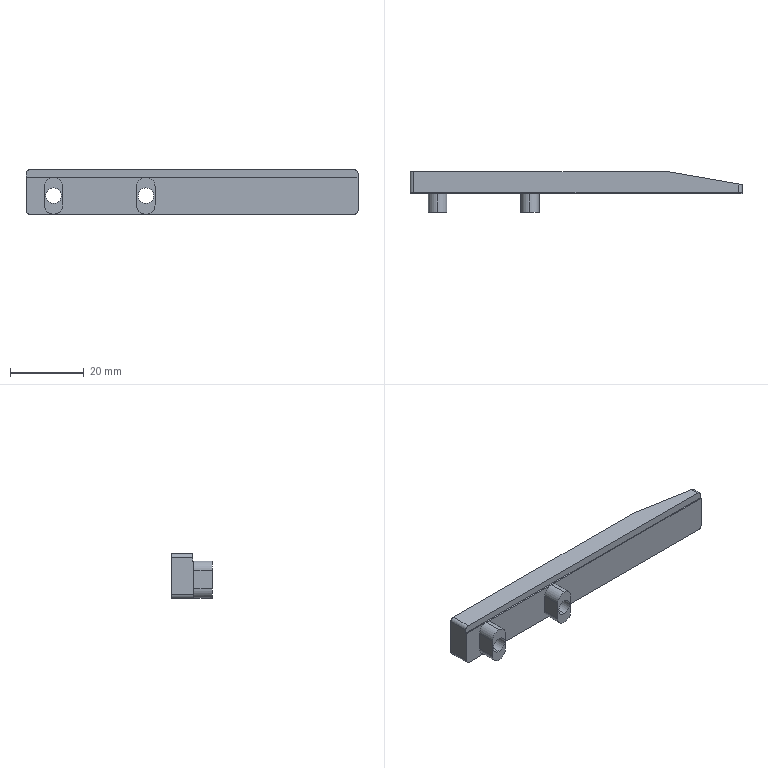Part | STEP file | 10000020548swp000-1 | 1 solid | 37 faces | box 90 x 11 x 12 mm | volume 5809 mm3 | plane 19 | cylinder 18 | commonest cylinder face diameters 5 x6 2 x4 4.2 x4 8 x4
STEP:
#1=CARTESIAN_POINT('',(7.5,1.4,-5.));
#2=VERTEX_POINT('',#1);
#3=CARTESIAN_POINT('',(7.5,1.4,3.));
#4=VERTEX_POINT('',#3);
#5=CARTESIAN_POINT('',(7.5,1.4,-1.));
#6=DIRECTION('',(0.,1.,0.));
#7=DIRECTION('',(0.,0.,1.));
#8=AXIS2_PLACEMENT_3D('',#5,#6,#7);
#9=CIRCLE('',#8,4.);
#10=EDGE_CURVE('',#2,#4,#9,.T.);
#11=ORIENTED_EDGE('',*,*,#10,.F.);
#12=CARTESIAN_POINT('',(7.5,6.,-5.));
#13=VERTEX_POINT('',#12);
#14=CARTESIAN_POINT('',(7.5,6.,-5.));
#15=DIRECTION('',(0.,1.,0.));
#16=VECTOR('',#15,1000.);
#17=LINE('',#14,#16);
#18=EDGE_CURVE('',#2,#13,#17,.T.);
#19=ORIENTED_EDGE('',*,*,#18,.T.);
#20=CARTESIAN_POINT('',(7.5,6.,3.));
#21=VERTEX_POINT('',#20);
#22=CARTESIAN_POINT('',(7.5,6.,-1.));
#23=DIRECTION('',(0.,1.,0.));
#24=DIRECTION('',(0.,0.,1.));
#25=AXIS2_PLACEMENT_3D('',#22,#23,#24);
#26=CIRCLE('',#25,4.);
#27=EDGE_CURVE('',#13,#21,#26,.T.);
#28=ORIENTED_EDGE('',*,*,#27,.T.);
#29=CARTESIAN_POINT('',(7.5,6.,3.));
#30=DIRECTION('',(0.,1.,0.));
#31=VECTOR('',#30,1000.);
#32=LINE('',#29,#31);
#33=EDGE_CURVE('',#4,#21,#32,.T.);
#34=ORIENTED_EDGE('',*,*,#33,.F.);
#35=EDGE_LOOP('',(#11,#19,#28,#34));
#36=FACE_OUTER_BOUND('',#35,.T.);
#37=CARTESIAN_POINT('',(7.5,6.,-1.));
#38=DIRECTION('',(0.,1.,0.));
#39=DIRECTION('',(0.,0.,1.));
#40=AXIS2_PLACEMENT_3D('',#37,#38,#39);
#41=CYLINDRICAL_SURFACE('',#40,4.);
#42=ADVANCED_FACE('',(#36),#41,.F.);
#43=CARTESIAN_POINT('',(7.5,-5.,1.1));
#44=VERTEX_POINT('',#43);
#45=CARTESIAN_POINT('',(7.5,-5.,-3.1));
#46=VERTEX_POINT('',#45);
#47=CARTESIAN_POINT('',(7.5,-5.,-1.));
#48=DIRECTION('',(0.,-1.,0.));
#49=DIRECTION('',(0.,0.,-1.));
#50=AXIS2_PLACEMENT_3D('',#47,#48,#49);
#51=CIRCLE('',#50,2.1);
#52=EDGE_CURVE('',#44,#46,#51,.T.);
#53=ORIENTED_EDGE('',*,*,#52,.T.);
#54=CARTESIAN_POINT('',(7.5,1.4,-3.1));
#55=VERTEX_POINT('',#54);
#56=CARTESIAN_POINT('',(7.5,6.,-3.1));
#57=DIRECTION('',(0.,1.,0.));
#58=VECTOR('',#57,1000.);
#59=LINE('',#56,#58);
#60=EDGE_CURVE('',#46,#55,#59,.T.);
#61=ORIENTED_EDGE('',*,*,#60,.T.);
#62=CARTESIAN_POINT('',(7.5,1.4,1.1));
#63=VERTEX_POINT('',#62);
#64=CARTESIAN_POINT('',(7.5,1.4,-1.));
#65=DIRECTION('',(0.,1.,0.));
#66=DIRECTION('',(0.,0.,1.));
#67=AXIS2_PLACEMENT_3D('',#64,#65,#66);
#68=CIRCLE('',#67,2.1);
#69=EDGE_CURVE('',#55,#63,#68,.T.);
#70=ORIENTED_EDGE('',*,*,#69,.T.);
#71=CARTESIAN_POINT('',(7.5,6.,1.1));
#72=DIRECTION('',(0.,1.,0.));
#73=VECTOR('',#72,1000.);
#74=LINE('',#71,#73);
#75=EDGE_CURVE('',#44,#63,#74,.T.);
#76=ORIENTED_EDGE('',*,*,#75,.F.);
#77=EDGE_LOOP('',(#53,#61,#70,#76));
#78=FACE_OUTER_BOUND('',#77,.T.);
#79=CARTESIAN_POINT('',(7.5,6.,-1.));
#80=DIRECTION('',(0.,1.,0.));
#81=DIRECTION('',(0.,0.,1.));
#82=AXIS2_PLACEMENT_3D('',#79,#80,#81);
#83=CYLINDRICAL_SURFACE('',#82,2.1);
#84=ADVANCED_FACE('',(#78),#83,.F.);
#85=CARTESIAN_POINT('',(32.5,1.4,-5.));
#86=VERTEX_POINT('',#85);
#87=CARTESIAN_POINT('',(32.5,1.4,3.));
#88=VERTEX_POINT('',#87);
#89=CARTESIAN_POINT('',(32.5,1.4,-1.));
#90=DIRECTION('',(0.,1.,0.));
#91=DIRECTION('',(0.,0.,1.));
#92=AXIS2_PLACEMENT_3D('',#89,#90,#91);
#93=CIRCLE('',#92,4.);
#94=EDGE_CURVE('',#86,#88,#93,.T.);
#95=ORIENTED_EDGE('',*,*,#94,.F.);
#96=CARTESIAN_POINT('',(32.5,6.,-5.));
#97=VERTEX_POINT('',#96);
#98=CARTESIAN_POINT('',(32.5,6.,-5.));
#99=DIRECTION('',(0.,1.,0.));
#100=VECTOR('',#99,1000.);
#101=LINE('',#98,#100);
#102=EDGE_CURVE('',#86,#97,#101,.T.);
#103=ORIENTED_EDGE('',*,*,#102,.T.);
#104=CARTESIAN_POINT('',(32.5,6.,3.));
#105=VERTEX_POINT('',#104);
#106=CARTESIAN_POINT('',(32.5,6.,-1.));
#107=DIRECTION('',(0.,1.,0.));
#108=DIRECTION('',(0.,0.,1.));
#109=AXIS2_PLACEMENT_3D('',#106,#107,#108);
#110=CIRCLE('',#109,4.);
#111=EDGE_CURVE('',#97,#105,#110,.T.);
#112=ORIENTED_EDGE('',*,*,#111,.T.);
#113=CARTESIAN_POINT('',(32.5,6.,3.));
#114=DIRECTION('',(0.,1.,0.));
#115=VECTOR('',#114,1000.);
#116=LINE('',#113,#115);
#117=EDGE_CURVE('',#88,#105,#116,.T.);
#118=ORIENTED_EDGE('',*,*,#117,.F.);
#119=EDGE_LOOP('',(#95,#103,#112,#118));
#120=FACE_OUTER_BOUND('',#119,.T.);
#121=CARTESIAN_POINT('',(32.5,6.,-1.));
#122=DIRECTION('',(0.,1.,0.));
#123=DIRECTION('',(0.,0.,1.));
#124=AXIS2_PLACEMENT_3D('',#121,#122,#123);
#125=CYLINDRICAL_SURFACE('',#124,4.);
#126=ADVANCED_FACE('',(#120),#125,.F.);
#127=CARTESIAN_POINT('',(32.5,-5.,1.1));
#128=VERTEX_POINT('',#127);
#129=CARTESIAN_POINT('',(32.5,-5.,-3.1));
#130=VERTEX_POINT('',#129);
#131=CARTESIAN_POINT('',(32.5,-5.,-1.));
#132=DIRECTION('',(0.,-1.,0.));
#133=DIRECTION('',(0.,0.,-1.));
#134=AXIS2_PLACEMENT_3D('',#131,#132,#133);
#135=CIRCLE('',#134,2.1);
#136=EDGE_CURVE('',#128,#130,#135,.T.);
#137=ORIENTED_EDGE('',*,*,#136,.T.);
#138=CARTESIAN_POINT('',(32.5,1.4,-3.1));
#139=VERTEX_POINT('',#138);
#140=CARTESIAN_POINT('',(32.5,6.,-3.1));
#141=DIRECTION('',(0.,1.,0.));
#142=VECTOR('',#141,1000.);
#143=LINE('',#140,#142);
#144=EDGE_CURVE('',#130,#139,#143,.T.);
#145=ORIENTED_EDGE('',*,*,#144,.T.);
#146=CARTESIAN_POINT('',(32.5,1.4,1.1));
#147=VERTEX_POINT('',#146);
#148=CARTESIAN_POINT('',(32.5,1.4,-1.));
#149=DIRECTION('',(0.,1.,0.));
#150=DIRECTION('',(0.,0.,1.));
#151=AXIS2_PLACEMENT_3D('',#148,#149,#150);
#152=CIRCLE('',#151,2.1);
#153=EDGE_CURVE('',#139,#147,#152,.T.);
#154=ORIENTED_EDGE('',*,*,#153,.T.);
#155=CARTESIAN_POINT('',(32.5,6.,1.1));
#156=DIRECTION('',(0.,1.,0.));
#157=VECTOR('',#156,1000.);
#158=LINE('',#155,#157);
#159=EDGE_CURVE('',#128,#147,#158,.T.);
#160=ORIENTED_EDGE('',*,*,#159,.F.);
#161=EDGE_LOOP('',(#137,#145,#154,#160));
#162=FACE_OUTER_BOUND('',#161,.T.);
#163=CARTESIAN_POINT('',(32.5,6.,-1.));
#164=DIRECTION('',(0.,1.,0.));
#165=DIRECTION('',(0.,0.,1.));
#166=AXIS2_PLACEMENT_3D('',#163,#164,#165);
#167=CYLINDRICAL_SURFACE('',#166,2.1);
#168=ADVANCED_FACE('',(#162),#167,.F.);
#169=CARTESIAN_POINT('',(32.5,-5.,4.));
#170=VERTEX_POINT('',#169);
#171=CARTESIAN_POINT('',(30.,-5.,1.5));
#172=VERTEX_POINT('',#171);
#173=CARTESIAN_POINT('',(32.5,-5.,1.5));
#174=DIRECTION('',(0.,-1.,0.));
#175=DIRECTION('',(0.,0.,-1.));
#176=AXIS2_PLACEMENT_3D('',#173,#174,#175);
#177=CIRCLE('',#176,2.5);
#178=EDGE_CURVE('',#170,#172,#177,.T.);
#179=ORIENTED_EDGE('',*,*,#178,.F.);
#180=CARTESIAN_POINT('',(32.5,0.,4.));
#181=VERTEX_POINT('',#180);
#182=CARTESIAN_POINT('',(32.5,-5.,4.));
#183=DIRECTION('',(0.,1.,0.));
#184=VECTOR('',#183,1000.);
#185=LINE('',#182,#184);
#186=EDGE_CURVE('',#170,#181,#185,.T.);
#187=ORIENTED_EDGE('',*,*,#186,.T.);
#188=CARTESIAN_POINT('',(30.,0.,1.5));
#189=VERTEX_POINT('',#188);
#190=CARTESIAN_POINT('',(32.5,0.,1.5));
#191=DIRECTION('',(0.,-1.,0.));
#192=DIRECTION('',(0.,0.,-1.));
#193=AXIS2_PLACEMENT_3D('',#190,#191,#192);
#194=CIRCLE('',#193,2.5);
#195=EDGE_CURVE('',#181,#189,#194,.T.);
#196=ORIENTED_EDGE('',*,*,#195,.T.);
#197=CARTESIAN_POINT('',(30.,-5.,1.5));
#198=DIRECTION('',(0.,1.,0.));
#199=VECTOR('',#198,1000.);
#200=LINE('',#197,#199);
#201=EDGE_CURVE('',#172,#189,#200,.T.);
#202=ORIENTED_EDGE('',*,*,#201,.F.);
#203=EDGE_LOOP('',(#179,#187,#196,#202));
#204=FACE_OUTER_BOUND('',#203,.T.);
#205=CARTESIAN_POINT('',(32.5,-5.,1.5));
#206=DIRECTION('',(0.,1.,0.));
#207=DIRECTION('',(0.,0.,1.));
#208=AXIS2_PLACEMENT_3D('',#205,#206,#207);
#209=CYLINDRICAL_SURFACE('',#208,2.5);
#210=ADVANCED_FACE('',(#204),#209,.T.);
#211=CARTESIAN_POINT('',(7.5,-5.,4.));
#212=VERTEX_POINT('',#211);
#213=CARTESIAN_POINT('',(5.,-5.,1.5));
#214=VERTEX_POINT('',#213);
#215=CARTESIAN_POINT('',(7.5,-5.,1.5));
#216=DIRECTION('',(0.,-1.,0.));
#217=DIRECTION('',(0.,0.,-1.));
#218=AXIS2_PLACEMENT_3D('',#215,#216,#217);
#219=CIRCLE('',#218,2.5);
#220=EDGE_CURVE('',#212,#214,#219,.T.);
#221=ORIENTED_EDGE('',*,*,#220,.F.);
#222=CARTESIAN_POINT('',(7.5,0.,4.));
#223=VERTEX_POINT('',#222);
#224=CARTESIAN_POINT('',(7.5,-5.,4.));
#225=DIRECTION('',(0.,1.,0.));
#226=VECTOR('',#225,1000.);
#227=LINE('',#224,#226);
#228=EDGE_CURVE('',#212,#223,#227,.T.);
#229=ORIENTED_EDGE('',*,*,#228,.T.);
#230=CARTESIAN_POINT('',(5.,0.,1.5));
#231=VERTEX_POINT('',#230);
#232=CARTESIAN_POINT('',(7.5,0.,1.5));
#233=DIRECTION('',(0.,-1.,0.));
#234=DIRECTION('',(0.,0.,-1.));
#235=AXIS2_PLACEMENT_3D('',#232,#233,#234);
#236=CIRCLE('',#235,2.5);
#237=EDGE_CURVE('',#223,#231,#236,.T.);
#238=ORIENTED_EDGE('',*,*,#237,.T.);
#239=CARTESIAN_POINT('',(5.,-5.,1.5));
#240=DIRECTION('',(0.,1.,0.));
#241=VECTOR('',#240,1000.);
#242=LINE('',#239,#241);
#243=EDGE_CURVE('',#214,#231,#242,.T.);
#244=ORIENTED_EDGE('',*,*,#243,.F.);
#245=EDGE_LOOP('',(#221,#229,#238,#244));
#246=FACE_OUTER_BOUND('',#245,.T.);
#247=CARTESIAN_POINT('',(7.5,-5.,1.5));
#248=DIRECTION('',(0.,1.,0.));
#249=DIRECTION('',(0.,0.,1.));
#250=AXIS2_PLACEMENT_3D('',#247,#248,#249);
#251=CYLINDRICAL_SURFACE('',#250,2.5);
#252=ADVANCED_FACE('',(#246),#251,.T.);
#253=CARTESIAN_POINT('',(32.5,0.,-6.));
#254=VERTEX_POINT('',#253);
#255=CARTESIAN_POINT('',(89.,0.,-6.));
#256=VERTEX_POINT('',#255);
#257=CARTESIAN_POINT('',(0.,0.,-6.));
#258=DIRECTION('',(1.,0.,0.));
#259=VECTOR('',#258,1000.);
#260=LINE('',#257,#259);
#261=EDGE_CURVE('',#254,#256,#260,.T.);
#262=ORIENTED_EDGE('',*,*,#261,.T.);
#263=CARTESIAN_POINT('',(90.,0.,-5.));
#264=VERTEX_POINT('',#263);
#265=CARTESIAN_POINT('',(89.,0.,-5.));
#266=DIRECTION('',(0.,-1.,0.));
#267=DIRECTION('',(0.,0.,1.));
#268=AXIS2_PLACEMENT_3D('',#265,#266,#267);
#269=CIRCLE('',#268,1.);
#270=EDGE_CURVE('',#256,#264,#269,.T.);
#271=ORIENTED_EDGE('',*,*,#270,.T.);
#272=CARTESIAN_POINT('',(90.,0.,4.));
#273=VERTEX_POINT('',#272);
#274=CARTESIAN_POINT('',(90.,0.,6.));
#275=DIRECTION('',(0.,0.,-1.));
#276=VECTOR('',#275,1000.);
#277=LINE('',#274,#276);
#278=EDGE_CURVE('',#273,#264,#277,.T.);
#279=ORIENTED_EDGE('',*,*,#278,.F.);
#280=CARTESIAN_POINT('',(90.,0.,4.));
#281=DIRECTION('',(1.,0.,0.));
#282=VECTOR('',#281,1000.);
#283=LINE('',#280,#282);
#284=EDGE_CURVE('',#181,#273,#283,.T.);
#285=ORIENTED_EDGE('',*,*,#284,.F.);
#286=CARTESIAN_POINT('',(35.,0.,1.5));
#287=VERTEX_POINT('',#286);
#288=CARTESIAN_POINT('',(32.5,0.,1.5));
#289=DIRECTION('',(0.,-1.,0.));
#290=DIRECTION('',(0.,0.,-1.));
#291=AXIS2_PLACEMENT_3D('',#288,#289,#290);
#292=CIRCLE('',#291,2.5);
#293=EDGE_CURVE('',#287,#181,#292,.T.);
#294=ORIENTED_EDGE('',*,*,#293,.F.);
#295=CARTESIAN_POINT('',(35.,0.,-3.5));
#296=VERTEX_POINT('',#295);
#297=CARTESIAN_POINT('',(35.,0.,1.5));
#298=DIRECTION('',(0.,0.,1.));
#299=VECTOR('',#298,1000.);
#300=LINE('',#297,#299);
#301=EDGE_CURVE('',#296,#287,#300,.T.);
#302=ORIENTED_EDGE('',*,*,#301,.F.);
#303=CARTESIAN_POINT('',(32.5,0.,-3.5));
#304=DIRECTION('',(0.,-1.,0.));
#305=DIRECTION('',(0.,0.,-1.));
#306=AXIS2_PLACEMENT_3D('',#303,#304,#305);
#307=CIRCLE('',#306,2.5);
#308=EDGE_CURVE('',#254,#296,#307,.T.);
#309=ORIENTED_EDGE('',*,*,#308,.F.);
#310=EDGE_LOOP('',(#262,#271,#279,#285,#294,#302,#309));
#311=FACE_OUTER_BOUND('',#310,.T.);
#312=CARTESIAN_POINT('',(0.,0.,6.));
#313=DIRECTION('',(0.,1.,0.));
#314=DIRECTION('',(0.,0.,1.));
#315=AXIS2_PLACEMENT_3D('',#312,#313,#314);
#316=PLANE('',#315);
#317=ADVANCED_FACE('',(#311),#316,.F.);
#318=ORIENTED_EDGE('',*,*,#195,.F.);
#319=CARTESIAN_POINT('',(90.,0.,4.));
#320=DIRECTION('',(1.,0.,0.));
#321=VECTOR('',#320,1000.);
#322=LINE('',#319,#321);
#323=EDGE_CURVE('',#223,#181,#322,.T.);
#324=ORIENTED_EDGE('',*,*,#323,.F.);
#325=CARTESIAN_POINT('',(10.,0.,1.5));
#326=VERTEX_POINT('',#325);
#327=CARTESIAN_POINT('',(7.5,0.,1.5));
#328=DIRECTION('',(0.,-1.,0.));
#329=DIRECTION('',(0.,0.,-1.));
#330=AXIS2_PLACEMENT_3D('',#327,#328,#329);
#331=CIRCLE('',#330,2.5);
#332=EDGE_CURVE('',#326,#223,#331,.T.);
#333=ORIENTED_EDGE('',*,*,#332,.F.);
#334=CARTESIAN_POINT('',(10.,0.,-3.5));
#335=VERTEX_POINT('',#334);
#336=CARTESIAN_POINT('',(10.,0.,1.5));
#337=DIRECTION('',(0.,0.,1.));
#338=VECTOR('',#337,1000.);
#339=LINE('',#336,#338);
#340=EDGE_CURVE('',#335,#326,#339,.T.);
#341=ORIENTED_EDGE('',*,*,#340,.F.);
#342=CARTESIAN_POINT('',(7.5,0.,-6.));
#343=VERTEX_POINT('',#342);
#344=CARTESIAN_POINT('',(7.5,0.,-3.5));
#345=DIRECTION('',(0.,-1.,0.));
#346=DIRECTION('',(0.,0.,-1.));
#347=AXIS2_PLACEMENT_3D('',#344,#345,#346);
#348=CIRCLE('',#347,2.5);
#349=EDGE_CURVE('',#343,#335,#348,.T.);
#350=ORIENTED_EDGE('',*,*,#349,.F.);
#351=CARTESIAN_POINT('',(0.,0.,-6.));
#352=DIRECTION('',(1.,0.,0.));
#353=VECTOR('',#352,1000.);
#354=LINE('',#351,#353);
#355=EDGE_CURVE('',#343,#254,#354,.T.);
#356=ORIENTED_EDGE('',*,*,#355,.T.);
#357=CARTESIAN_POINT('',(30.,0.,-3.5));
#358=VERTEX_POINT('',#357);
#359=CARTESIAN_POINT('',(32.5,0.,-3.5));
#360=DIRECTION('',(0.,-1.,0.));
#361=DIRECTION('',(0.,0.,-1.));
#362=AXIS2_PLACEMENT_3D('',#359,#360,#361);
#363=CIRCLE('',#362,2.5);
#364=EDGE_CURVE('',#358,#254,#363,.T.);
#365=ORIENTED_EDGE('',*,*,#364,.F.);
#366=CARTESIAN_POINT('',(30.,0.,1.5));
#367=DIRECTION('',(0.,0.,-1.));
#368=VECTOR('',#367,1000.);
#369=LINE('',#366,#368);
#370=EDGE_CURVE('',#189,#358,#369,.T.);
#371=ORIENTED_EDGE('',*,*,#370,.F.);
#372=EDGE_LOOP('',(#318,#324,#333,#341,#350,#356,#365,#371));
#373=FACE_OUTER_BOUND('',#372,.T.);
#374=CARTESIAN_POINT('',(0.,0.,6.));
#375=DIRECTION('',(0.,1.,0.));
#376=DIRECTION('',(0.,0.,1.));
#377=AXIS2_PLACEMENT_3D('',#374,#375,#376);
#378=PLANE('',#377);
#379=ADVANCED_FACE('',(#373),#378,.F.);
#380=CARTESIAN_POINT('',(0.,0.,4.));
#381=VERTEX_POINT('',#380);
#382=CARTESIAN_POINT('',(0.,0.,-5.));
#383=VERTEX_POINT('',#382);
#384=CARTESIAN_POINT('',(0.,0.,6.));
#385=DIRECTION('',(0.,0.,-1.));
#386=VECTOR('',#385,1000.);
#387=LINE('',#384,#386);
#388=EDGE_CURVE('',#381,#383,#387,.T.);
#389=ORIENTED_EDGE('',*,*,#388,.T.);
#390=CARTESIAN_POINT('',(1.,0.,-6.));
#391=VERTEX_POINT('',#390);
#392=CARTESIAN_POINT('',(1.,0.,-5.));
#393=DIRECTION('',(0.,-1.,0.));
#394=DIRECTION('',(0.,0.,1.));
#395=AXIS2_PLACEMENT_3D('',#392,#393,#394);
#396=CIRCLE('',#395,1.);
#397=EDGE_CURVE('',#383,#391,#396,.T.);
#398=ORIENTED_EDGE('',*,*,#397,.T.);
#399=CARTESIAN_POINT('',(0.,0.,-6.));
#400=DIRECTION('',(1.,0.,0.));
#401=VECTOR('',#400,1000.);
#402=LINE('',#399,#401);
#403=EDGE_CURVE('',#391,#343,#402,.T.);
#404=ORIENTED_EDGE('',*,*,#403,.T.);
#405=CARTESIAN_POINT('',(5.,0.,-3.5));
#406=VERTEX_POINT('',#405);
#407=CARTESIAN_POINT('',(7.5,0.,-3.5));
#408=DIRECTION('',(0.,-1.,0.));
#409=DIRECTION('',(0.,0.,-1.));
#410=AXIS2_PLACEMENT_3D('',#407,#408,#409);
#411=CIRCLE('',#410,2.5);
#412=EDGE_CURVE('',#406,#343,#411,.T.);
#413=ORIENTED_EDGE('',*,*,#412,.F.);
#414=CARTESIAN_POINT('',(5.,0.,1.5));
#415=DIRECTION('',(0.,0.,-1.));
#416=VECTOR('',#415,1000.);
#417=LINE('',#414,#416);
#418=EDGE_CURVE('',#231,#406,#417,.T.);
#419=ORIENTED_EDGE('',*,*,#418,.F.);
#420=ORIENTED_EDGE('',*,*,#237,.F.);
#421=CARTESIAN_POINT('',(90.,0.,4.));
#422=DIRECTION('',(1.,0.,0.));
#423=VECTOR('',#422,1000.);
#424=LINE('',#421,#423);
#425=EDGE_CURVE('',#381,#223,#424,.T.);
#426=ORIENTED_EDGE('',*,*,#425,.F.);
#427=EDGE_LOOP('',(#389,#398,#404,#413,#419,#420,#426));
#428=FACE_OUTER_BOUND('',#427,.T.);
#429=CARTESIAN_POINT('',(0.,0.,6.));
#430=DIRECTION('',(0.,1.,0.));
#431=DIRECTION('',(0.,0.,1.));
#432=AXIS2_PLACEMENT_3D('',#429,#430,#431);
#433=PLANE('',#432);
#434=ADVANCED_FACE('',(#428),#433,.F.);
#435=CARTESIAN_POINT('',(0.,6.,5.));
#436=VERTEX_POINT('',#435);
#437=CARTESIAN_POINT('',(0.,6.,-5.));
#438=VERTEX_POINT('',#437);
#439=CARTESIAN_POINT('',(0.,6.,6.));
#440=DIRECTION('',(0.,0.,-1.));
#441=VECTOR('',#440,1000.);
#442=LINE('',#439,#441);
#443=EDGE_CURVE('',#436,#438,#442,.T.);
#444=ORIENTED_EDGE('',*,*,#443,.T.);
#445=CARTESIAN_POINT('',(0.,0.,-5.));
#446=DIRECTION('',(0.,-1.,0.));
#447=VECTOR('',#446,1000.);
#448=LINE('',#445,#447);
#449=EDGE_CURVE('',#438,#383,#448,.T.);
#450=ORIENTED_EDGE('',*,*,#449,.T.);
#451=ORIENTED_EDGE('',*,*,#388,.F.);
#452=CARTESIAN_POINT('',(0.,0.3,4.));
#453=VERTEX_POINT('',#452);
#454=CARTESIAN_POINT('',(0.,0.,4.));
#455=DIRECTION('',(0.,-1.,0.));
#456=VECTOR('',#455,1000.);
#457=LINE('',#454,#456);
#458=EDGE_CURVE('',#453,#381,#457,.T.);
#459=ORIENTED_EDGE('',*,*,#458,.F.);
#460=CARTESIAN_POINT('',(0.,0.3,5.));
#461=VERTEX_POINT('',#460);
#462=CARTESIAN_POINT('',(0.,0.3,4.));
#463=DIRECTION('',(0.,0.,1.));
#464=VECTOR('',#463,1000.);
#465=LINE('',#462,#464);
#466=EDGE_CURVE('',#453,#461,#465,.T.);
#467=ORIENTED_EDGE('',*,*,#466,.T.);
#468=CARTESIAN_POINT('',(0.,0.,5.));
#469=DIRECTION('',(0.,1.,0.));
#470=VECTOR('',#469,1000.);
#471=LINE('',#468,#470);
#472=EDGE_CURVE('',#461,#436,#471,.T.);
#473=ORIENTED_EDGE('',*,*,#472,.T.);
#474=EDGE_LOOP('',(#444,#450,#451,#459,#467,#473));
#475=FACE_OUTER_BOUND('',#474,.T.);
#476=CARTESIAN_POINT('',(0.,0.,6.));
#477=DIRECTION('',(1.,0.,0.));
#478=DIRECTION('',(0.,0.,-1.));
#479=AXIS2_PLACEMENT_3D('',#476,#477,#478);
#480=PLANE('',#479);
#481=ADVANCED_FACE('',(#475),#480,.F.);
#482=ORIENTED_EDGE('',*,*,#278,.T.);
#483=CARTESIAN_POINT('',(90.,2.5,-5.));
#484=VERTEX_POINT('',#483);
#485=CARTESIAN_POINT('',(90.,2.5,-5.));
#486=DIRECTION('',(0.,1.,0.));
#487=VECTOR('',#486,1000.);
#488=LINE('',#485,#487);
#489=EDGE_CURVE('',#264,#484,#488,.T.);
#490=ORIENTED_EDGE('',*,*,#489,.T.);
#491=CARTESIAN_POINT('',(90.,2.5,5.));
#492=VERTEX_POINT('',#491);
#493=CARTESIAN_POINT('',(90.,2.5,6.));
#494=DIRECTION('',(0.,0.,-1.));
#495=VECTOR('',#494,1000.);
#496=LINE('',#493,#495);
#497=EDGE_CURVE('',#492,#484,#496,.T.);
#498=ORIENTED_EDGE('',*,*,#497,.F.);
#499=CARTESIAN_POINT('',(90.,0.3,5.));
#500=VERTEX_POINT('',#499);
#501=CARTESIAN_POINT('',(90.,0.,5.));
#502=DIRECTION('',(0.,-1.,0.));
#503=VECTOR('',#502,1000.);
#504=LINE('',#501,#503);
#505=EDGE_CURVE('',#492,#500,#504,.T.);
#506=ORIENTED_EDGE('',*,*,#505,.T.);
#507=CARTESIAN_POINT('',(90.,0.3,4.));
#508=VERTEX_POINT('',#507);
#509=CARTESIAN_POINT('',(90.,0.3,4.));
#510=DIRECTION('',(0.,0.,1.));
#511=VECTOR('',#510,1000.);
#512=LINE('',#509,#511);
#513=EDGE_CURVE('',#508,#500,#512,.T.);
#514=ORIENTED_EDGE('',*,*,#513,.F.);
#515=CARTESIAN_POINT('',(90.,0.,4.));
#516=DIRECTION('',(0.,1.,0.));
#517=VECTOR('',#516,1000.);
#518=LINE('',#515,#517);
#519=EDGE_CURVE('',#273,#508,#518,.T.);
#520=ORIENTED_EDGE('',*,*,#519,.F.);
#521=EDGE_LOOP('',(#482,#490,#498,#506,#514,#520));
#522=FACE_OUTER_BOUND('',#521,.T.);
#523=CARTESIAN_POINT('',(90.,0.,6.));
#524=DIRECTION('',(-1.,0.,0.));
#525=DIRECTION('',(0.,0.,1.));
#526=AXIS2_PLACEMENT_3D('',#523,#524,#525);
#527=PLANE('',#526);
#528=ADVANCED_FACE('',(#522),#527,.F.);
#529=ORIENTED_EDGE('',*,*,#497,.T.);
#530=CARTESIAN_POINT('',(89.,2.675,-6.));
#531=VERTEX_POINT('',#530);
#532=CARTESIAN_POINT('',(90.,2.5,-5.));
#533=CARTESIAN_POINT('',(90.,2.5,-5.586));
#534=CARTESIAN_POINT('',(89.586,2.572,-6.));
#535=CARTESIAN_POINT('',(89.,2.675,-6.));
#536=(BOUNDED_CURVE()B_SPLINE_CURVE(3,(#532,#533,#534,#535),.UNSPECIFIED.,.F.,.F.)B_SPLINE_CURVE_WITH_KNOTS((4,4),(0.,1.571),.UNSPECIFIED.)CURVE()GEOMETRIC_REPRESENTATION_ITEM()RATIONAL_B_SPLINE_CURVE((1.,0.8047,0.8047,1.))REPRESENTATION_ITEM(''));
#537=EDGE_CURVE('',#484,#531,#536,.T.);
#538=ORIENTED_EDGE('',*,*,#537,.T.);
#539=CARTESIAN_POINT('',(70.,6.,-6.));
#540=VERTEX_POINT('',#539);
#541=CARTESIAN_POINT('',(90.,2.5,-6.));
#542=DIRECTION('',(-0.985,0.1724,0.));
#543=VECTOR('',#542,1000.);
#544=LINE('',#541,#543);
#545=EDGE_CURVE('',#531,#540,#544,.T.);
#546=ORIENTED_EDGE('',*,*,#545,.T.);
#547=CARTESIAN_POINT('',(70.,6.,6.));
#548=VERTEX_POINT('',#547);
#549=CARTESIAN_POINT('',(70.,6.,6.));
#550=DIRECTION('',(0.,0.,-1.));
#551=VECTOR('',#550,1000.);
#552=LINE('',#549,#551);
#553=EDGE_CURVE('',#548,#540,#552,.T.);
#554=ORIENTED_EDGE('',*,*,#553,.F.);
#555=CARTESIAN_POINT('',(89.,2.675,6.));
#556=VERTEX_POINT('',#555);
#557=CARTESIAN_POINT('',(90.,2.5,6.));
#558=DIRECTION('',(-0.985,0.1724,0.));
#559=VECTOR('',#558,1000.);
#560=LINE('',#557,#559);
#561=EDGE_CURVE('',#556,#548,#560,.T.);
#562=ORIENTED_EDGE('',*,*,#561,.F.);
#563=CARTESIAN_POINT('',(89.,2.675,6.));
#564=CARTESIAN_POINT('',(89.586,2.572,6.));
#565=CARTESIAN_POINT('',(90.,2.5,5.586));
#566=CARTESIAN_POINT('',(90.,2.5,5.));
#567=(BOUNDED_CURVE()B_SPLINE_CURVE(3,(#563,#564,#565,#566),.UNSPECIFIED.,.F.,.F.)B_SPLINE_CURVE_WITH_KNOTS((4,4),(1.571,3.142),.UNSPECIFIED.)CURVE()GEOMETRIC_REPRESENTATION_ITEM()RATIONAL_B_SPLINE_CURVE((1.,0.8047,0.8047,1.))REPRESENTATION_ITEM(''));
#568=EDGE_CURVE('',#556,#492,#567,.T.);
#569=ORIENTED_EDGE('',*,*,#568,.T.);
#570=EDGE_LOOP('',(#529,#538,#546,#554,#562,#569));
#571=FACE_OUTER_BOUND('',#570,.T.);
#572=CARTESIAN_POINT('',(90.,2.5,6.));
#573=DIRECTION('',(-0.1724,-0.985,0.));
#574=DIRECTION('',(0.985,-0.1724,0.));
#575=AXIS2_PLACEMENT_3D('',#572,#573,#574);
#576=PLANE('',#575);
#577=ADVANCED_FACE('',(#571),#576,.F.);
#578=CARTESIAN_POINT('',(7.5,6.,-1.));
#579=DIRECTION('',(0.,1.,0.));
#580=DIRECTION('',(0.,0.,1.));
#581=AXIS2_PLACEMENT_3D('',#578,#579,#580);
#582=CIRCLE('',#581,4.);
#583=EDGE_CURVE('',#21,#13,#582,.T.);
#584=ORIENTED_EDGE('',*,*,#583,.F.);
#585=ORIENTED_EDGE('',*,*,#27,.F.);
#586=EDGE_LOOP('',(#584,#585));
#587=FACE_BOUND('',#586,.T.);
#588=CARTESIAN_POINT('',(32.5,6.,-1.));
#589=DIRECTION('',(0.,1.,0.));
#590=DIRECTION('',(0.,0.,1.));
#591=AXIS2_PLACEMENT_3D('',#588,#589,#590);
#592=CIRCLE('',#591,4.);
#593=EDGE_CURVE('',#105,#97,#592,.T.);
#594=ORIENTED_EDGE('',*,*,#593,.F.);
#595=ORIENTED_EDGE('',*,*,#111,.F.);
#596=EDGE_LOOP('',(#594,#595));
#597=FACE_BOUND('',#596,.T.);
#598=CARTESIAN_POINT('',(1.,6.,-6.));
#599=VERTEX_POINT('',#598);
#600=CARTESIAN_POINT('',(0.,6.,-6.));
#601=DIRECTION('',(-1.,0.,0.));
#602=VECTOR('',#601,1000.);
#603=LINE('',#600,#602);
#604=EDGE_CURVE('',#540,#599,#603,.T.);
#605=ORIENTED_EDGE('',*,*,#604,.T.);
#606=CARTESIAN_POINT('',(1.,6.,-5.));
#607=DIRECTION('',(0.,1.,0.));
#608=DIRECTION('',(0.,0.,-1.));
#609=AXIS2_PLACEMENT_3D('',#606,#607,#608);
#610=CIRCLE('',#609,1.);
#611=EDGE_CURVE('',#599,#438,#610,.T.);
#612=ORIENTED_EDGE('',*,*,#611,.T.);
#613=ORIENTED_EDGE('',*,*,#443,.F.);
#614=CARTESIAN_POINT('',(1.,6.,6.));
#615=VERTEX_POINT('',#614);
#616=CARTESIAN_POINT('',(1.,6.,5.));
#617=DIRECTION('',(0.,1.,0.));
#618=DIRECTION('',(0.,0.,-1.));
#619=AXIS2_PLACEMENT_3D('',#616,#617,#618);
#620=CIRCLE('',#619,1.);
#621=EDGE_CURVE('',#436,#615,#620,.T.);
#622=ORIENTED_EDGE('',*,*,#621,.T.);
#623=CARTESIAN_POINT('',(0.,6.,6.));
#624=DIRECTION('',(-1.,0.,0.));
#625=VECTOR('',#624,1000.);
#626=LINE('',#623,#625);
#627=EDGE_CURVE('',#548,#615,#626,.T.);
#628=ORIENTED_EDGE('',*,*,#627,.F.);
#629=ORIENTED_EDGE('',*,*,#553,.T.);
#630=EDGE_LOOP('',(#605,#612,#613,#622,#628,#629));
#631=FACE_OUTER_BOUND('',#630,.T.);
#632=CARTESIAN_POINT('',(0.,6.,6.));
#633=DIRECTION('',(0.,-1.,0.));
#634=DIRECTION('',(0.,0.,-1.));
#635=AXIS2_PLACEMENT_3D('',#632,#633,#634);
#636=PLANE('',#635);
#637=ADVANCED_FACE('',(#587,#597,#631),#636,.F.);
#638=ORIENTED_EDGE('',*,*,#627,.T.);
#639=CARTESIAN_POINT('',(1.,0.3,6.));
#640=VERTEX_POINT('',#639);
#641=CARTESIAN_POINT('',(1.,0.,6.));
#642=DIRECTION('',(0.,-1.,0.));
#643=VECTOR('',#642,1000.);
#644=LINE('',#641,#643);
#645=EDGE_CURVE('',#615,#640,#644,.T.);
#646=ORIENTED_EDGE('',*,*,#645,.T.);
#647=CARTESIAN_POINT('',(89.,0.3,6.));
#648=VERTEX_POINT('',#647);
#649=CARTESIAN_POINT('',(90.,0.3,6.));
#650=DIRECTION('',(-1.,0.,0.));
#651=VECTOR('',#650,1000.);
#652=LINE('',#649,#651);
#653=EDGE_CURVE('',#648,#640,#652,.T.);
#654=ORIENTED_EDGE('',*,*,#653,.F.);
#655=CARTESIAN_POINT('',(89.,0.,6.));
#656=DIRECTION('',(0.,1.,0.));
#657=VECTOR('',#656,1000.);
#658=LINE('',#655,#657);
#659=EDGE_CURVE('',#648,#556,#658,.T.);
#660=ORIENTED_EDGE('',*,*,#659,.T.);
#661=ORIENTED_EDGE('',*,*,#561,.T.);
#662=EDGE_LOOP('',(#638,#646,#654,#660,#661));
#663=FACE_OUTER_BOUND('',#662,.T.);
#664=CARTESIAN_POINT('',(0.,0.,6.));
#665=DIRECTION('',(0.,0.,-1.));
#666=DIRECTION('',(-1.,0.,0.));
#667=AXIS2_PLACEMENT_3D('',#664,#665,#666);
#668=PLANE('',#667);
#669=ADVANCED_FACE('',(#663),#668,.F.);
#670=ORIENTED_EDGE('',*,*,#403,.F.);
#671=CARTESIAN_POINT('',(1.,6.,-6.));
#672=DIRECTION('',(0.,1.,0.));
#673=VECTOR('',#672,1000.);
#674=LINE('',#671,#673);
#675=EDGE_CURVE('',#391,#599,#674,.T.);
#676=ORIENTED_EDGE('',*,*,#675,.T.);
#677=ORIENTED_EDGE('',*,*,#604,.F.);
#678=ORIENTED_EDGE('',*,*,#545,.F.);
#679=CARTESIAN_POINT('',(89.,0.,-6.));
#680=DIRECTION('',(0.,-1.,0.));
#681=VECTOR('',#680,1000.);
#682=LINE('',#679,#681);
#683=EDGE_CURVE('',#531,#256,#682,.T.);
#684=ORIENTED_EDGE('',*,*,#683,.T.);
#685=ORIENTED_EDGE('',*,*,#261,.F.);
#686=ORIENTED_EDGE('',*,*,#355,.F.);
#687=EDGE_LOOP('',(#670,#676,#677,#678,#684,#685,#686));
#688=FACE_OUTER_BOUND('',#687,.T.);
#689=CARTESIAN_POINT('',(0.,0.,-6.));
#690=DIRECTION('',(0.,0.,-1.));
#691=DIRECTION('',(-1.,0.,0.));
#692=AXIS2_PLACEMENT_3D('',#689,#690,#691);
#693=PLANE('',#692);
#694=ADVANCED_FACE('',(#688),#693,.T.);
#695=ORIENTED_EDGE('',*,*,#653,.T.);
#696=CARTESIAN_POINT('',(1.,0.3,5.));
#697=DIRECTION('',(0.,-1.,0.));
#698=DIRECTION('',(-1.,0.,0.));
#699=AXIS2_PLACEMENT_3D('',#696,#697,#698);
#700=CIRCLE('',#699,1.);
#701=EDGE_CURVE('',#640,#461,#700,.T.);
#702=ORIENTED_EDGE('',*,*,#701,.T.);
#703=ORIENTED_EDGE('',*,*,#466,.F.);
#704=CARTESIAN_POINT('',(90.,0.3,4.));
#705=DIRECTION('',(-1.,0.,0.));
#706=VECTOR('',#705,1000.);
#707=LINE('',#704,#706);
#708=EDGE_CURVE('',#508,#453,#707,.T.);
#709=ORIENTED_EDGE('',*,*,#708,.F.);
#710=ORIENTED_EDGE('',*,*,#513,.T.);
#711=CARTESIAN_POINT('',(89.,0.3,5.));
#712=DIRECTION('',(0.,-1.,0.));
#713=DIRECTION('',(-1.,0.,0.));
#714=AXIS2_PLACEMENT_3D('',#711,#712,#713);
#715=CIRCLE('',#714,1.);
#716=EDGE_CURVE('',#500,#648,#715,.T.);
#717=ORIENTED_EDGE('',*,*,#716,.T.);
#718=EDGE_LOOP('',(#695,#702,#703,#709,#710,#717));
#719=FACE_OUTER_BOUND('',#718,.T.);
#720=CARTESIAN_POINT('',(90.,0.3,4.));
#721=DIRECTION('',(0.,1.,0.));
#722=DIRECTION('',(-1.,0.,0.));
#723=AXIS2_PLACEMENT_3D('',#720,#721,#722);
#724=PLANE('',#723);
#725=ADVANCED_FACE('',(#719),#724,.F.);
#726=ORIENTED_EDGE('',*,*,#519,.T.);
#727=ORIENTED_EDGE('',*,*,#708,.T.);
#728=ORIENTED_EDGE('',*,*,#458,.T.);
#729=ORIENTED_EDGE('',*,*,#425,.T.);
#730=ORIENTED_EDGE('',*,*,#323,.T.);
#731=ORIENTED_EDGE('',*,*,#284,.T.);
#732=EDGE_LOOP('',(#726,#727,#728,#729,#730,#731));
#733=FACE_OUTER_BOUND('',#732,.T.);
#734=CARTESIAN_POINT('',(0.,0.,4.));
#735=DIRECTION('',(0.,0.,1.));
#736=DIRECTION('',(1.,0.,0.));
#737=AXIS2_PLACEMENT_3D('',#734,#735,#736);
#738=PLANE('',#737);
#739=ADVANCED_FACE('',(#733),#738,.T.);
#740=ORIENTED_EDGE('',*,*,#228,.F.);
#741=CARTESIAN_POINT('',(10.,-5.,1.5));
#742=VERTEX_POINT('',#741);
#743=CARTESIAN_POINT('',(7.5,-5.,1.5));
#744=DIRECTION('',(0.,-1.,0.));
#745=DIRECTION('',(0.,0.,-1.));
#746=AXIS2_PLACEMENT_3D('',#743,#744,#745);
#747=CIRCLE('',#746,2.5);
#748=EDGE_CURVE('',#742,#212,#747,.T.);
#749=ORIENTED_EDGE('',*,*,#748,.F.);
#750=CARTESIAN_POINT('',(10.,-5.,1.5));
#751=DIRECTION('',(0.,1.,0.));
#752=VECTOR('',#751,1000.);
#753=LINE('',#750,#752);
#754=EDGE_CURVE('',#742,#326,#753,.T.);
#755=ORIENTED_EDGE('',*,*,#754,.T.);
#756=ORIENTED_EDGE('',*,*,#332,.T.);
#757=EDGE_LOOP('',(#740,#749,#755,#756));
#758=FACE_OUTER_BOUND('',#757,.T.);
#759=CARTESIAN_POINT('',(7.5,-5.,1.5));
#760=DIRECTION('',(0.,1.,0.));
#761=DIRECTION('',(0.,0.,1.));
#762=AXIS2_PLACEMENT_3D('',#759,#760,#761);
#763=CYLINDRICAL_SURFACE('',#762,2.5);
#764=ADVANCED_FACE('',(#758),#763,.T.);
#765=ORIENTED_EDGE('',*,*,#418,.T.);
#766=CARTESIAN_POINT('',(5.,-5.,-3.5));
#767=VERTEX_POINT('',#766);
#768=CARTESIAN_POINT('',(5.,-5.,-3.5));
#769=DIRECTION('',(0.,1.,0.));
#770=VECTOR('',#769,1000.);
#771=LINE('',#768,#770);
#772=EDGE_CURVE('',#767,#406,#771,.T.);
#773=ORIENTED_EDGE('',*,*,#772,.F.);
#774=CARTESIAN_POINT('',(5.,-5.,1.5));
#775=DIRECTION('',(0.,0.,-1.));
#776=VECTOR('',#775,1000.);
#777=LINE('',#774,#776);
#778=EDGE_CURVE('',#214,#767,#777,.T.);
#779=ORIENTED_EDGE('',*,*,#778,.F.);
#780=ORIENTED_EDGE('',*,*,#243,.T.);
#781=EDGE_LOOP('',(#765,#773,#779,#780));
#782=FACE_OUTER_BOUND('',#781,.T.);
#783=CARTESIAN_POINT('',(5.,-5.,1.5));
#784=DIRECTION('',(1.,0.,0.));
#785=DIRECTION('',(0.,0.,-1.));
#786=AXIS2_PLACEMENT_3D('',#783,#784,#785);
#787=PLANE('',#786);
#788=ADVANCED_FACE('',(#782),#787,.F.);
#789=ORIENTED_EDGE('',*,*,#412,.T.);
#790=ORIENTED_EDGE('',*,*,#349,.T.);
#791=CARTESIAN_POINT('',(10.,-5.,-3.5));
#792=VERTEX_POINT('',#791);
#793=CARTESIAN_POINT('',(10.,-5.,-3.5));
#794=DIRECTION('',(0.,1.,0.));
#795=VECTOR('',#794,1000.);
#796=LINE('',#793,#795);
#797=EDGE_CURVE('',#792,#335,#796,.T.);
#798=ORIENTED_EDGE('',*,*,#797,.F.);
#799=CARTESIAN_POINT('',(7.5,-5.,-3.5));
#800=DIRECTION('',(0.,-1.,0.));
#801=DIRECTION('',(0.,0.,-1.));
#802=AXIS2_PLACEMENT_3D('',#799,#800,#801);
#803=CIRCLE('',#802,2.5);
#804=EDGE_CURVE('',#767,#792,#803,.T.);
#805=ORIENTED_EDGE('',*,*,#804,.F.);
#806=ORIENTED_EDGE('',*,*,#772,.T.);
#807=EDGE_LOOP('',(#789,#790,#798,#805,#806));
#808=FACE_OUTER_BOUND('',#807,.T.);
#809=CARTESIAN_POINT('',(7.5,-5.,-3.5));
#810=DIRECTION('',(0.,1.,0.));
#811=DIRECTION('',(0.,0.,1.));
#812=AXIS2_PLACEMENT_3D('',#809,#810,#811);
#813=CYLINDRICAL_SURFACE('',#812,2.5);
#814=ADVANCED_FACE('',(#808),#813,.T.);
#815=ORIENTED_EDGE('',*,*,#340,.T.);
#816=ORIENTED_EDGE('',*,*,#754,.F.);
#817=CARTESIAN_POINT('',(10.,-5.,1.5));
#818=DIRECTION('',(0.,0.,1.));
#819=VECTOR('',#818,1000.);
#820=LINE('',#817,#819);
#821=EDGE_CURVE('',#792,#742,#820,.T.);
#822=ORIENTED_EDGE('',*,*,#821,.F.);
#823=ORIENTED_EDGE('',*,*,#797,.T.);
#824=EDGE_LOOP('',(#815,#816,#822,#823));
#825=FACE_OUTER_BOUND('',#824,.T.);
#826=CARTESIAN_POINT('',(10.,-5.,1.5));
#827=DIRECTION('',(-1.,0.,0.));
#828=DIRECTION('',(0.,0.,1.));
#829=AXIS2_PLACEMENT_3D('',#826,#827,#828);
#830=PLANE('',#829);
#831=ADVANCED_FACE('',(#825),#830,.F.);
#832=ORIENTED_EDGE('',*,*,#52,.F.);
#833=CARTESIAN_POINT('',(7.5,-5.,-1.));
#834=DIRECTION('',(0.,-1.,0.));
#835=DIRECTION('',(0.,0.,-1.));
#836=AXIS2_PLACEMENT_3D('',#833,#834,#835);
#837=CIRCLE('',#836,2.1);
#838=EDGE_CURVE('',#46,#44,#837,.T.);
#839=ORIENTED_EDGE('',*,*,#838,.F.);
#840=EDGE_LOOP('',(#832,#839));
#841=FACE_BOUND('',#840,.T.);
#842=ORIENTED_EDGE('',*,*,#748,.T.);
#843=ORIENTED_EDGE('',*,*,#220,.T.);
#844=ORIENTED_EDGE('',*,*,#778,.T.);
#845=ORIENTED_EDGE('',*,*,#804,.T.);
#846=ORIENTED_EDGE('',*,*,#821,.T.);
#847=EDGE_LOOP('',(#842,#843,#844,#845,#846));
#848=FACE_OUTER_BOUND('',#847,.T.);
#849=CARTESIAN_POINT('',(7.5,-5.,1.5));
#850=DIRECTION('',(0.,-1.,0.));
#851=DIRECTION('',(0.,0.,-1.));
#852=AXIS2_PLACEMENT_3D('',#849,#850,#851);
#853=PLANE('',#852);
#854=ADVANCED_FACE('',(#841,#848),#853,.T.);
#855=ORIENTED_EDGE('',*,*,#186,.F.);
#856=CARTESIAN_POINT('',(35.,-5.,1.5));
#857=VERTEX_POINT('',#856);
#858=CARTESIAN_POINT('',(32.5,-5.,1.5));
#859=DIRECTION('',(0.,-1.,0.));
#860=DIRECTION('',(0.,0.,-1.));
#861=AXIS2_PLACEMENT_3D('',#858,#859,#860);
#862=CIRCLE('',#861,2.5);
#863=EDGE_CURVE('',#857,#170,#862,.T.);
#864=ORIENTED_EDGE('',*,*,#863,.F.);
#865=CARTESIAN_POINT('',(35.,-5.,1.5));
#866=DIRECTION('',(0.,1.,0.));
#867=VECTOR('',#866,1000.);
#868=LINE('',#865,#867);
#869=EDGE_CURVE('',#857,#287,#868,.T.);
#870=ORIENTED_EDGE('',*,*,#869,.T.);
#871=ORIENTED_EDGE('',*,*,#293,.T.);
#872=EDGE_LOOP('',(#855,#864,#870,#871));
#873=FACE_OUTER_BOUND('',#872,.T.);
#874=CARTESIAN_POINT('',(32.5,-5.,1.5));
#875=DIRECTION('',(0.,1.,0.));
#876=DIRECTION('',(0.,0.,1.));
#877=AXIS2_PLACEMENT_3D('',#874,#875,#876);
#878=CYLINDRICAL_SURFACE('',#877,2.5);
#879=ADVANCED_FACE('',(#873),#878,.T.);
#880=ORIENTED_EDGE('',*,*,#370,.T.);
#881=CARTESIAN_POINT('',(30.,-5.,-3.5));
#882=VERTEX_POINT('',#881);
#883=CARTESIAN_POINT('',(30.,-5.,-3.5));
#884=DIRECTION('',(0.,1.,0.));
#885=VECTOR('',#884,1000.);
#886=LINE('',#883,#885);
#887=EDGE_CURVE('',#882,#358,#886,.T.);
#888=ORIENTED_EDGE('',*,*,#887,.F.);
#889=CARTESIAN_POINT('',(30.,-5.,1.5));
#890=DIRECTION('',(0.,0.,-1.));
#891=VECTOR('',#890,1000.);
#892=LINE('',#889,#891);
#893=EDGE_CURVE('',#172,#882,#892,.T.);
#894=ORIENTED_EDGE('',*,*,#893,.F.);
#895=ORIENTED_EDGE('',*,*,#201,.T.);
#896=EDGE_LOOP('',(#880,#888,#894,#895));
#897=FACE_OUTER_BOUND('',#896,.T.);
#898=CARTESIAN_POINT('',(30.,-5.,1.5));
#899=DIRECTION('',(1.,0.,0.));
#900=DIRECTION('',(0.,0.,-1.));
#901=AXIS2_PLACEMENT_3D('',#898,#899,#900);
#902=PLANE('',#901);
#903=ADVANCED_FACE('',(#897),#902,.F.);
#904=ORIENTED_EDGE('',*,*,#364,.T.);
#905=ORIENTED_EDGE('',*,*,#308,.T.);
#906=CARTESIAN_POINT('',(35.,-5.,-3.5));
#907=VERTEX_POINT('',#906);
#908=CARTESIAN_POINT('',(35.,-5.,-3.5));
#909=DIRECTION('',(0.,1.,0.));
#910=VECTOR('',#909,1000.);
#911=LINE('',#908,#910);
#912=EDGE_CURVE('',#907,#296,#911,.T.);
#913=ORIENTED_EDGE('',*,*,#912,.F.);
#914=CARTESIAN_POINT('',(32.5,-5.,-3.5));
#915=DIRECTION('',(0.,-1.,0.));
#916=DIRECTION('',(0.,0.,-1.));
#917=AXIS2_PLACEMENT_3D('',#914,#915,#916);
#918=CIRCLE('',#917,2.5);
#919=EDGE_CURVE('',#882,#907,#918,.T.);
#920=ORIENTED_EDGE('',*,*,#919,.F.);
#921=ORIENTED_EDGE('',*,*,#887,.T.);
#922=EDGE_LOOP('',(#904,#905,#913,#920,#921));
#923=FACE_OUTER_BOUND('',#922,.T.);
#924=CARTESIAN_POINT('',(32.5,-5.,-3.5));
#925=DIRECTION('',(0.,1.,0.));
#926=DIRECTION('',(0.,0.,1.));
#927=AXIS2_PLACEMENT_3D('',#924,#925,#926);
#928=CYLINDRICAL_SURFACE('',#927,2.5);
#929=ADVANCED_FACE('',(#923),#928,.T.);
#930=ORIENTED_EDGE('',*,*,#301,.T.);
#931=ORIENTED_EDGE('',*,*,#869,.F.);
#932=CARTESIAN_POINT('',(35.,-5.,1.5));
#933=DIRECTION('',(0.,0.,1.));
#934=VECTOR('',#933,1000.);
#935=LINE('',#932,#934);
#936=EDGE_CURVE('',#907,#857,#935,.T.);
#937=ORIENTED_EDGE('',*,*,#936,.F.);
#938=ORIENTED_EDGE('',*,*,#912,.T.);
#939=EDGE_LOOP('',(#930,#931,#937,#938));
#940=FACE_OUTER_BOUND('',#939,.T.);
#941=CARTESIAN_POINT('',(35.,-5.,1.5));
#942=DIRECTION('',(-1.,0.,0.));
#943=DIRECTION('',(0.,0.,1.));
#944=AXIS2_PLACEMENT_3D('',#941,#942,#943);
#945=PLANE('',#944);
#946=ADVANCED_FACE('',(#940),#945,.F.);
#947=ORIENTED_EDGE('',*,*,#136,.F.);
#948=CARTESIAN_POINT('',(32.5,-5.,-1.));
#949=DIRECTION('',(0.,-1.,0.));
#950=DIRECTION('',(0.,0.,-1.));
#951=AXIS2_PLACEMENT_3D('',#948,#949,#950);
#952=CIRCLE('',#951,2.1);
#953=EDGE_CURVE('',#130,#128,#952,.T.);
#954=ORIENTED_EDGE('',*,*,#953,.F.);
#955=EDGE_LOOP('',(#947,#954));
#956=FACE_BOUND('',#955,.T.);
#957=ORIENTED_EDGE('',*,*,#863,.T.);
#958=ORIENTED_EDGE('',*,*,#178,.T.);
#959=ORIENTED_EDGE('',*,*,#893,.T.);
#960=ORIENTED_EDGE('',*,*,#919,.T.);
#961=ORIENTED_EDGE('',*,*,#936,.T.);
#962=EDGE_LOOP('',(#957,#958,#959,#960,#961));
#963=FACE_OUTER_BOUND('',#962,.T.);
#964=CARTESIAN_POINT('',(32.5,-5.,1.5));
#965=DIRECTION('',(0.,-1.,0.));
#966=DIRECTION('',(0.,0.,-1.));
#967=AXIS2_PLACEMENT_3D('',#964,#965,#966);
#968=PLANE('',#967);
#969=ADVANCED_FACE('',(#956,#963),#968,.T.);
#970=ORIENTED_EDGE('',*,*,#144,.F.);
#971=ORIENTED_EDGE('',*,*,#953,.T.);
#972=ORIENTED_EDGE('',*,*,#159,.T.);
#973=CARTESIAN_POINT('',(32.5,1.4,-1.));
#974=DIRECTION('',(0.,1.,0.));
#975=DIRECTION('',(0.,0.,1.));
#976=AXIS2_PLACEMENT_3D('',#973,#974,#975);
#977=CIRCLE('',#976,2.1);
#978=EDGE_CURVE('',#147,#139,#977,.T.);
#979=ORIENTED_EDGE('',*,*,#978,.T.);
#980=EDGE_LOOP('',(#970,#971,#972,#979));
#981=FACE_OUTER_BOUND('',#980,.T.);
#982=CARTESIAN_POINT('',(32.5,6.,-1.));
#983=DIRECTION('',(0.,1.,0.));
#984=DIRECTION('',(0.,0.,1.));
#985=AXIS2_PLACEMENT_3D('',#982,#983,#984);
#986=CYLINDRICAL_SURFACE('',#985,2.1);
#987=ADVANCED_FACE('',(#981),#986,.F.);
#988=ORIENTED_EDGE('',*,*,#978,.F.);
#989=ORIENTED_EDGE('',*,*,#153,.F.);
#990=EDGE_LOOP('',(#988,#989));
#991=FACE_BOUND('',#990,.T.);
#992=CARTESIAN_POINT('',(32.5,1.4,-1.));
#993=DIRECTION('',(0.,1.,0.));
#994=DIRECTION('',(0.,0.,1.));
#995=AXIS2_PLACEMENT_3D('',#992,#993,#994);
#996=CIRCLE('',#995,4.);
#997=EDGE_CURVE('',#88,#86,#996,.T.);
#998=ORIENTED_EDGE('',*,*,#997,.T.);
#999=ORIENTED_EDGE('',*,*,#94,.T.);
#1000=EDGE_LOOP('',(#998,#999));
#1001=FACE_OUTER_BOUND('',#1000,.T.);
#1002=CARTESIAN_POINT('',(34.6,1.4,-1.));
#1003=DIRECTION('',(0.,-1.,0.));
#1004=DIRECTION('',(0.,0.,-1.));
#1005=AXIS2_PLACEMENT_3D('',#1002,#1003,#1004);
#1006=PLANE('',#1005);
#1007=ADVANCED_FACE('',(#991,#1001),#1006,.F.);
#1008=ORIENTED_EDGE('',*,*,#102,.F.);
#1009=ORIENTED_EDGE('',*,*,#997,.F.);
#1010=ORIENTED_EDGE('',*,*,#117,.T.);
#1011=ORIENTED_EDGE('',*,*,#593,.T.);
#1012=EDGE_LOOP('',(#1008,#1009,#1010,#1011));
#1013=FACE_OUTER_BOUND('',#1012,.T.);
#1014=CARTESIAN_POINT('',(32.5,6.,-1.));
#1015=DIRECTION('',(0.,1.,0.));
#1016=DIRECTION('',(0.,0.,1.));
#1017=AXIS2_PLACEMENT_3D('',#1014,#1015,#1016);
#1018=CYLINDRICAL_SURFACE('',#1017,4.);
#1019=ADVANCED_FACE('',(#1013),#1018,.F.);
#1020=ORIENTED_EDGE('',*,*,#60,.F.);
#1021=ORIENTED_EDGE('',*,*,#838,.T.);
#1022=ORIENTED_EDGE('',*,*,#75,.T.);
#1023=CARTESIAN_POINT('',(7.5,1.4,-1.));
#1024=DIRECTION('',(0.,1.,0.));
#1025=DIRECTION('',(0.,0.,1.));
#1026=AXIS2_PLACEMENT_3D('',#1023,#1024,#1025);
#1027=CIRCLE('',#1026,2.1);
#1028=EDGE_CURVE('',#63,#55,#1027,.T.);
#1029=ORIENTED_EDGE('',*,*,#1028,.T.);
#1030=EDGE_LOOP('',(#1020,#1021,#1022,#1029));
#1031=FACE_OUTER_BOUND('',#1030,.T.);
#1032=CARTESIAN_POINT('',(7.5,6.,-1.));
#1033=DIRECTION('',(0.,1.,0.));
#1034=DIRECTION('',(0.,0.,1.));
#1035=AXIS2_PLACEMENT_3D('',#1032,#1033,#1034);
#1036=CYLINDRICAL_SURFACE('',#1035,2.1);
#1037=ADVANCED_FACE('',(#1031),#1036,.F.);
#1038=ORIENTED_EDGE('',*,*,#1028,.F.);
#1039=ORIENTED_EDGE('',*,*,#69,.F.);
#1040=EDGE_LOOP('',(#1038,#1039));
#1041=FACE_BOUND('',#1040,.T.);
#1042=CARTESIAN_POINT('',(7.5,1.4,-1.));
#1043=DIRECTION('',(0.,1.,0.));
#1044=DIRECTION('',(0.,0.,1.));
#1045=AXIS2_PLACEMENT_3D('',#1042,#1043,#1044);
#1046=CIRCLE('',#1045,4.);
#1047=EDGE_CURVE('',#4,#2,#1046,.T.);
#1048=ORIENTED_EDGE('',*,*,#1047,.T.);
#1049=ORIENTED_EDGE('',*,*,#10,.T.);
#1050=EDGE_LOOP('',(#1048,#1049));
#1051=FACE_OUTER_BOUND('',#1050,.T.);
#1052=CARTESIAN_POINT('',(9.6,1.4,-1.));
#1053=DIRECTION('',(0.,-1.,0.));
#1054=DIRECTION('',(0.,0.,-1.));
#1055=AXIS2_PLACEMENT_3D('',#1052,#1053,#1054);
#1056=PLANE('',#1055);
#1057=ADVANCED_FACE('',(#1041,#1051),#1056,.F.);
#1058=ORIENTED_EDGE('',*,*,#18,.F.);
#1059=ORIENTED_EDGE('',*,*,#1047,.F.);
#1060=ORIENTED_EDGE('',*,*,#33,.T.);
#1061=ORIENTED_EDGE('',*,*,#583,.T.);
#1062=EDGE_LOOP('',(#1058,#1059,#1060,#1061));
#1063=FACE_OUTER_BOUND('',#1062,.T.);
#1064=CARTESIAN_POINT('',(7.5,6.,-1.));
#1065=DIRECTION('',(0.,1.,0.));
#1066=DIRECTION('',(0.,0.,1.));
#1067=AXIS2_PLACEMENT_3D('',#1064,#1065,#1066);
#1068=CYLINDRICAL_SURFACE('',#1067,4.);
#1069=ADVANCED_FACE('',(#1063),#1068,.F.);
#1070=ORIENTED_EDGE('',*,*,#611,.F.);
#1071=ORIENTED_EDGE('',*,*,#675,.F.);
#1072=ORIENTED_EDGE('',*,*,#397,.F.);
#1073=ORIENTED_EDGE('',*,*,#449,.F.);
#1074=EDGE_LOOP('',(#1070,#1071,#1072,#1073));
#1075=FACE_OUTER_BOUND('',#1074,.T.);
#1076=CARTESIAN_POINT('',(1.,0.,-5.));
#1077=DIRECTION('',(0.,1.,0.));
#1078=DIRECTION('',(0.,0.,1.));
#1079=AXIS2_PLACEMENT_3D('',#1076,#1077,#1078);
#1080=CYLINDRICAL_SURFACE('',#1079,1.);
#1081=ADVANCED_FACE('',(#1075),#1080,.T.);
#1082=ORIENTED_EDGE('',*,*,#621,.F.);
#1083=ORIENTED_EDGE('',*,*,#472,.F.);
#1084=ORIENTED_EDGE('',*,*,#701,.F.);
#1085=ORIENTED_EDGE('',*,*,#645,.F.);
#1086=EDGE_LOOP('',(#1082,#1083,#1084,#1085));
#1087=FACE_OUTER_BOUND('',#1086,.T.);
#1088=CARTESIAN_POINT('',(1.,0.,5.));
#1089=DIRECTION('',(0.,-1.,0.));
#1090=DIRECTION('',(0.,0.,-1.));
#1091=AXIS2_PLACEMENT_3D('',#1088,#1089,#1090);
#1092=CYLINDRICAL_SURFACE('',#1091,1.);
#1093=ADVANCED_FACE('',(#1087),#1092,.T.);
#1094=ORIENTED_EDGE('',*,*,#270,.F.);
#1095=ORIENTED_EDGE('',*,*,#683,.F.);
#1096=ORIENTED_EDGE('',*,*,#537,.F.);
#1097=ORIENTED_EDGE('',*,*,#489,.F.);
#1098=EDGE_LOOP('',(#1094,#1095,#1096,#1097));
#1099=FACE_OUTER_BOUND('',#1098,.T.);
#1100=CARTESIAN_POINT('',(89.,0.,-5.));
#1101=DIRECTION('',(0.,-1.,0.));
#1102=DIRECTION('',(0.,0.,-1.));
#1103=AXIS2_PLACEMENT_3D('',#1100,#1101,#1102);
#1104=CYLINDRICAL_SURFACE('',#1103,1.);
#1105=ADVANCED_FACE('',(#1099),#1104,.T.);
#1106=ORIENTED_EDGE('',*,*,#716,.F.);
#1107=ORIENTED_EDGE('',*,*,#505,.F.);
#1108=ORIENTED_EDGE('',*,*,#568,.F.);
#1109=ORIENTED_EDGE('',*,*,#659,.F.);
#1110=EDGE_LOOP('',(#1106,#1107,#1108,#1109));
#1111=FACE_OUTER_BOUND('',#1110,.T.);
#1112=CARTESIAN_POINT('',(89.,0.,5.));
#1113=DIRECTION('',(0.,1.,0.));
#1114=DIRECTION('',(0.,0.,1.));
#1115=AXIS2_PLACEMENT_3D('',#1112,#1113,#1114);
#1116=CYLINDRICAL_SURFACE('',#1115,1.);
#1117=ADVANCED_FACE('',(#1111),#1116,.T.);
#1118=CLOSED_SHELL('',(#42,#84,#126,#168,#210,#252,#317,#379,#434,#481,#528,#577,#637,#669,#694,#725,#739,#764,#788,#814,#831,#854,#879,#903,#929,#946,#969,#987,#1007,#1019,#1037,#1057,#1069,#1081,#1093,#1105,#1117));
#1119=MANIFOLD_SOLID_BREP('',#1118);
#1120=CARTESIAN_POINT('',(0.,0.,0.));
#1121=DIRECTION('',(0.,0.,1.));
#1122=DIRECTION('',(1.,0.,0.));
#1123=AXIS2_PLACEMENT_3D('',#1120,#1121,#1122);
#1124=(LENGTH_UNIT()NAMED_UNIT(*)SI_UNIT(.MILLI.,.METRE.));
#1125=UNCERTAINTY_MEASURE_WITH_UNIT(LENGTH_MEASURE(0.00001),#1124,'','');
#1126=(NAMED_UNIT(*)PLANE_ANGLE_UNIT()SI_UNIT($,.RADIAN.));
#1127=(NAMED_UNIT(*)SI_UNIT($,.STERADIAN.)SOLID_ANGLE_UNIT());
#1128=(GEOMETRIC_REPRESENTATION_CONTEXT(3)GLOBAL_UNCERTAINTY_ASSIGNED_CONTEXT((#1125))GLOBAL_UNIT_ASSIGNED_CONTEXT((#1124,#1126,#1127))REPRESENTATION_CONTEXT('',''));
#1129=ADVANCED_BREP_SHAPE_REPRESENTATION('',(#1119,#1123),#1128);